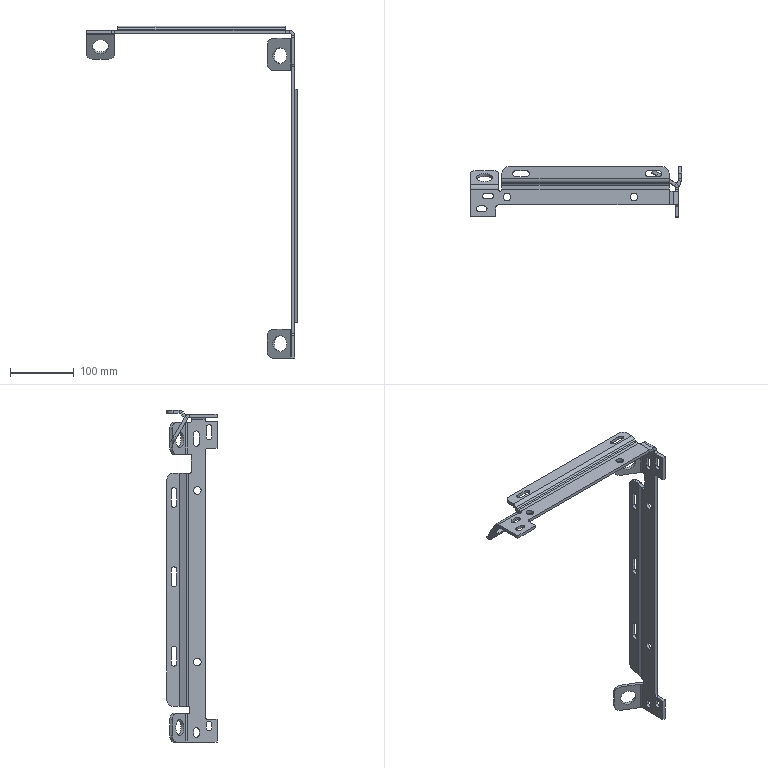Part | STEP file | 68352819 | 1 solid | 181 faces | box 333 x 78.764 x 522.5 mm | volume 245441 mm3 | plane 106 | cylinder 75 | commonest cylinder face diameters 9 x24 20 x10 5 x9 6 x9 12 x8 16 x8